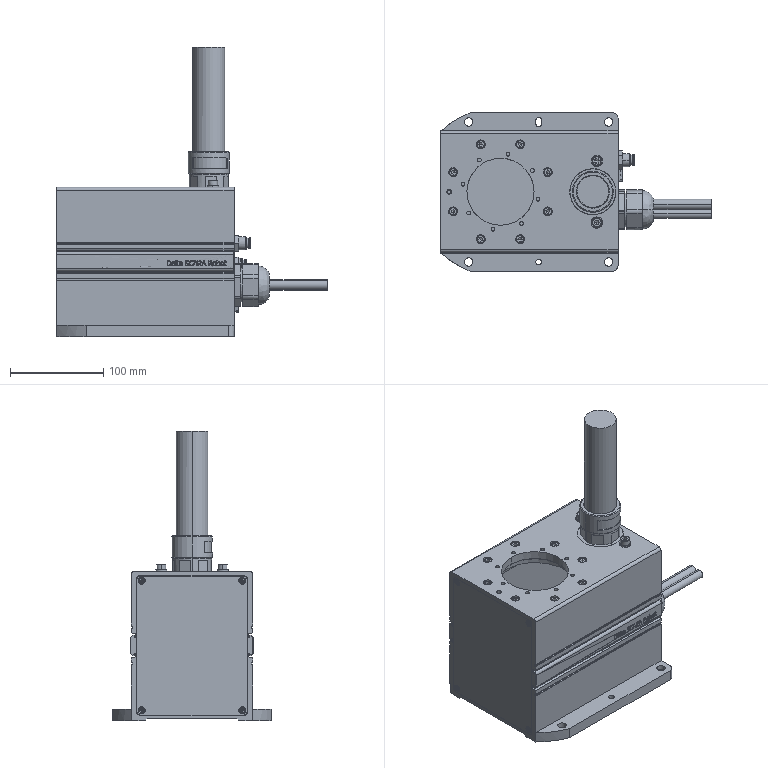Part | STEP file | 11-Base1111 | 19 solids | 1688 faces | box 290.067 x 170 x 310 mm | volume 1578242 mm3 | plane 845 | cylinder 465 | spline 192 | cone 154 | torus 32 | commonest cylinder face diameters 1 x76 6 x50 4.134 x32 5 x26 2.459 x20 4 x17